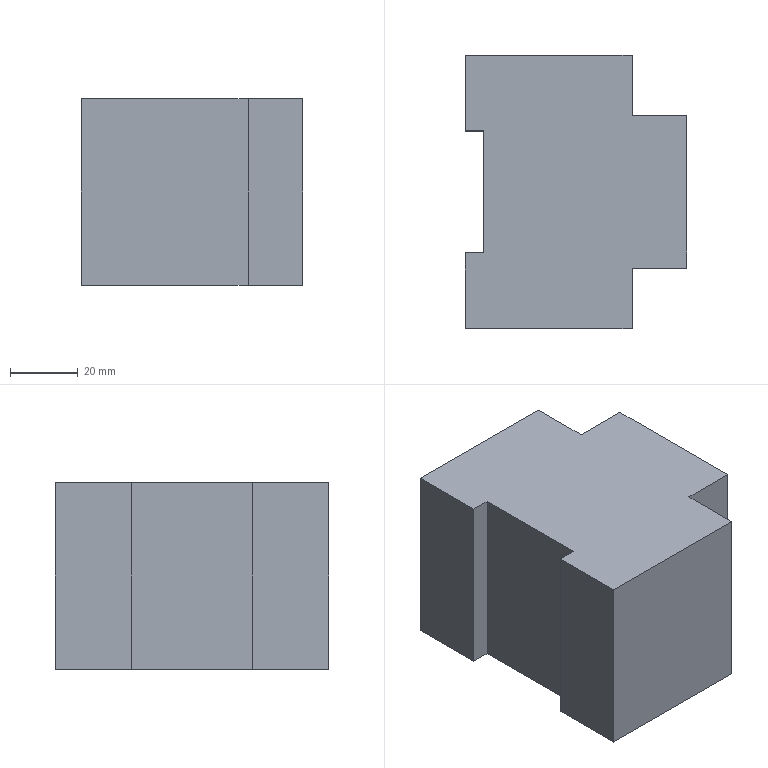Part | STEP file | Rail socket EA9XN310 | 1 solid | 29 faces | box 65.5 x 80.8 x 55 mm | volume 247844 mm3 | plane 29